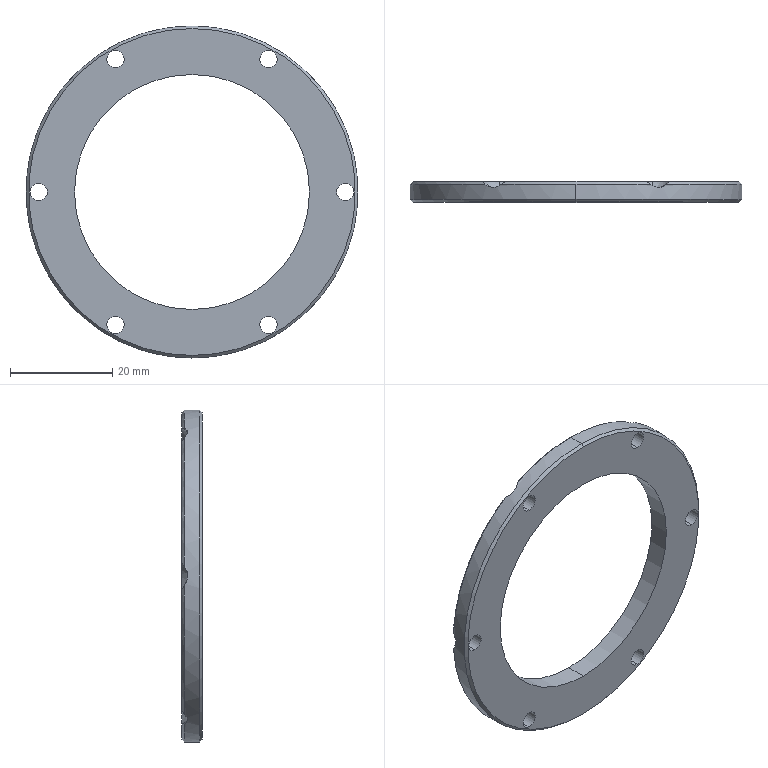Part | SolidWorks | features Chamfer 1, Extrusion 1, HoleWzd 1 | 1 solid | 45 faces | box 65 x 4 x 65 mm | volume 6250 mm3 | cone 21 | cylinder 16 | spline 6 | plane 2 | commonest cylinder face diameters 3.4 x12 46 x2 65 x2